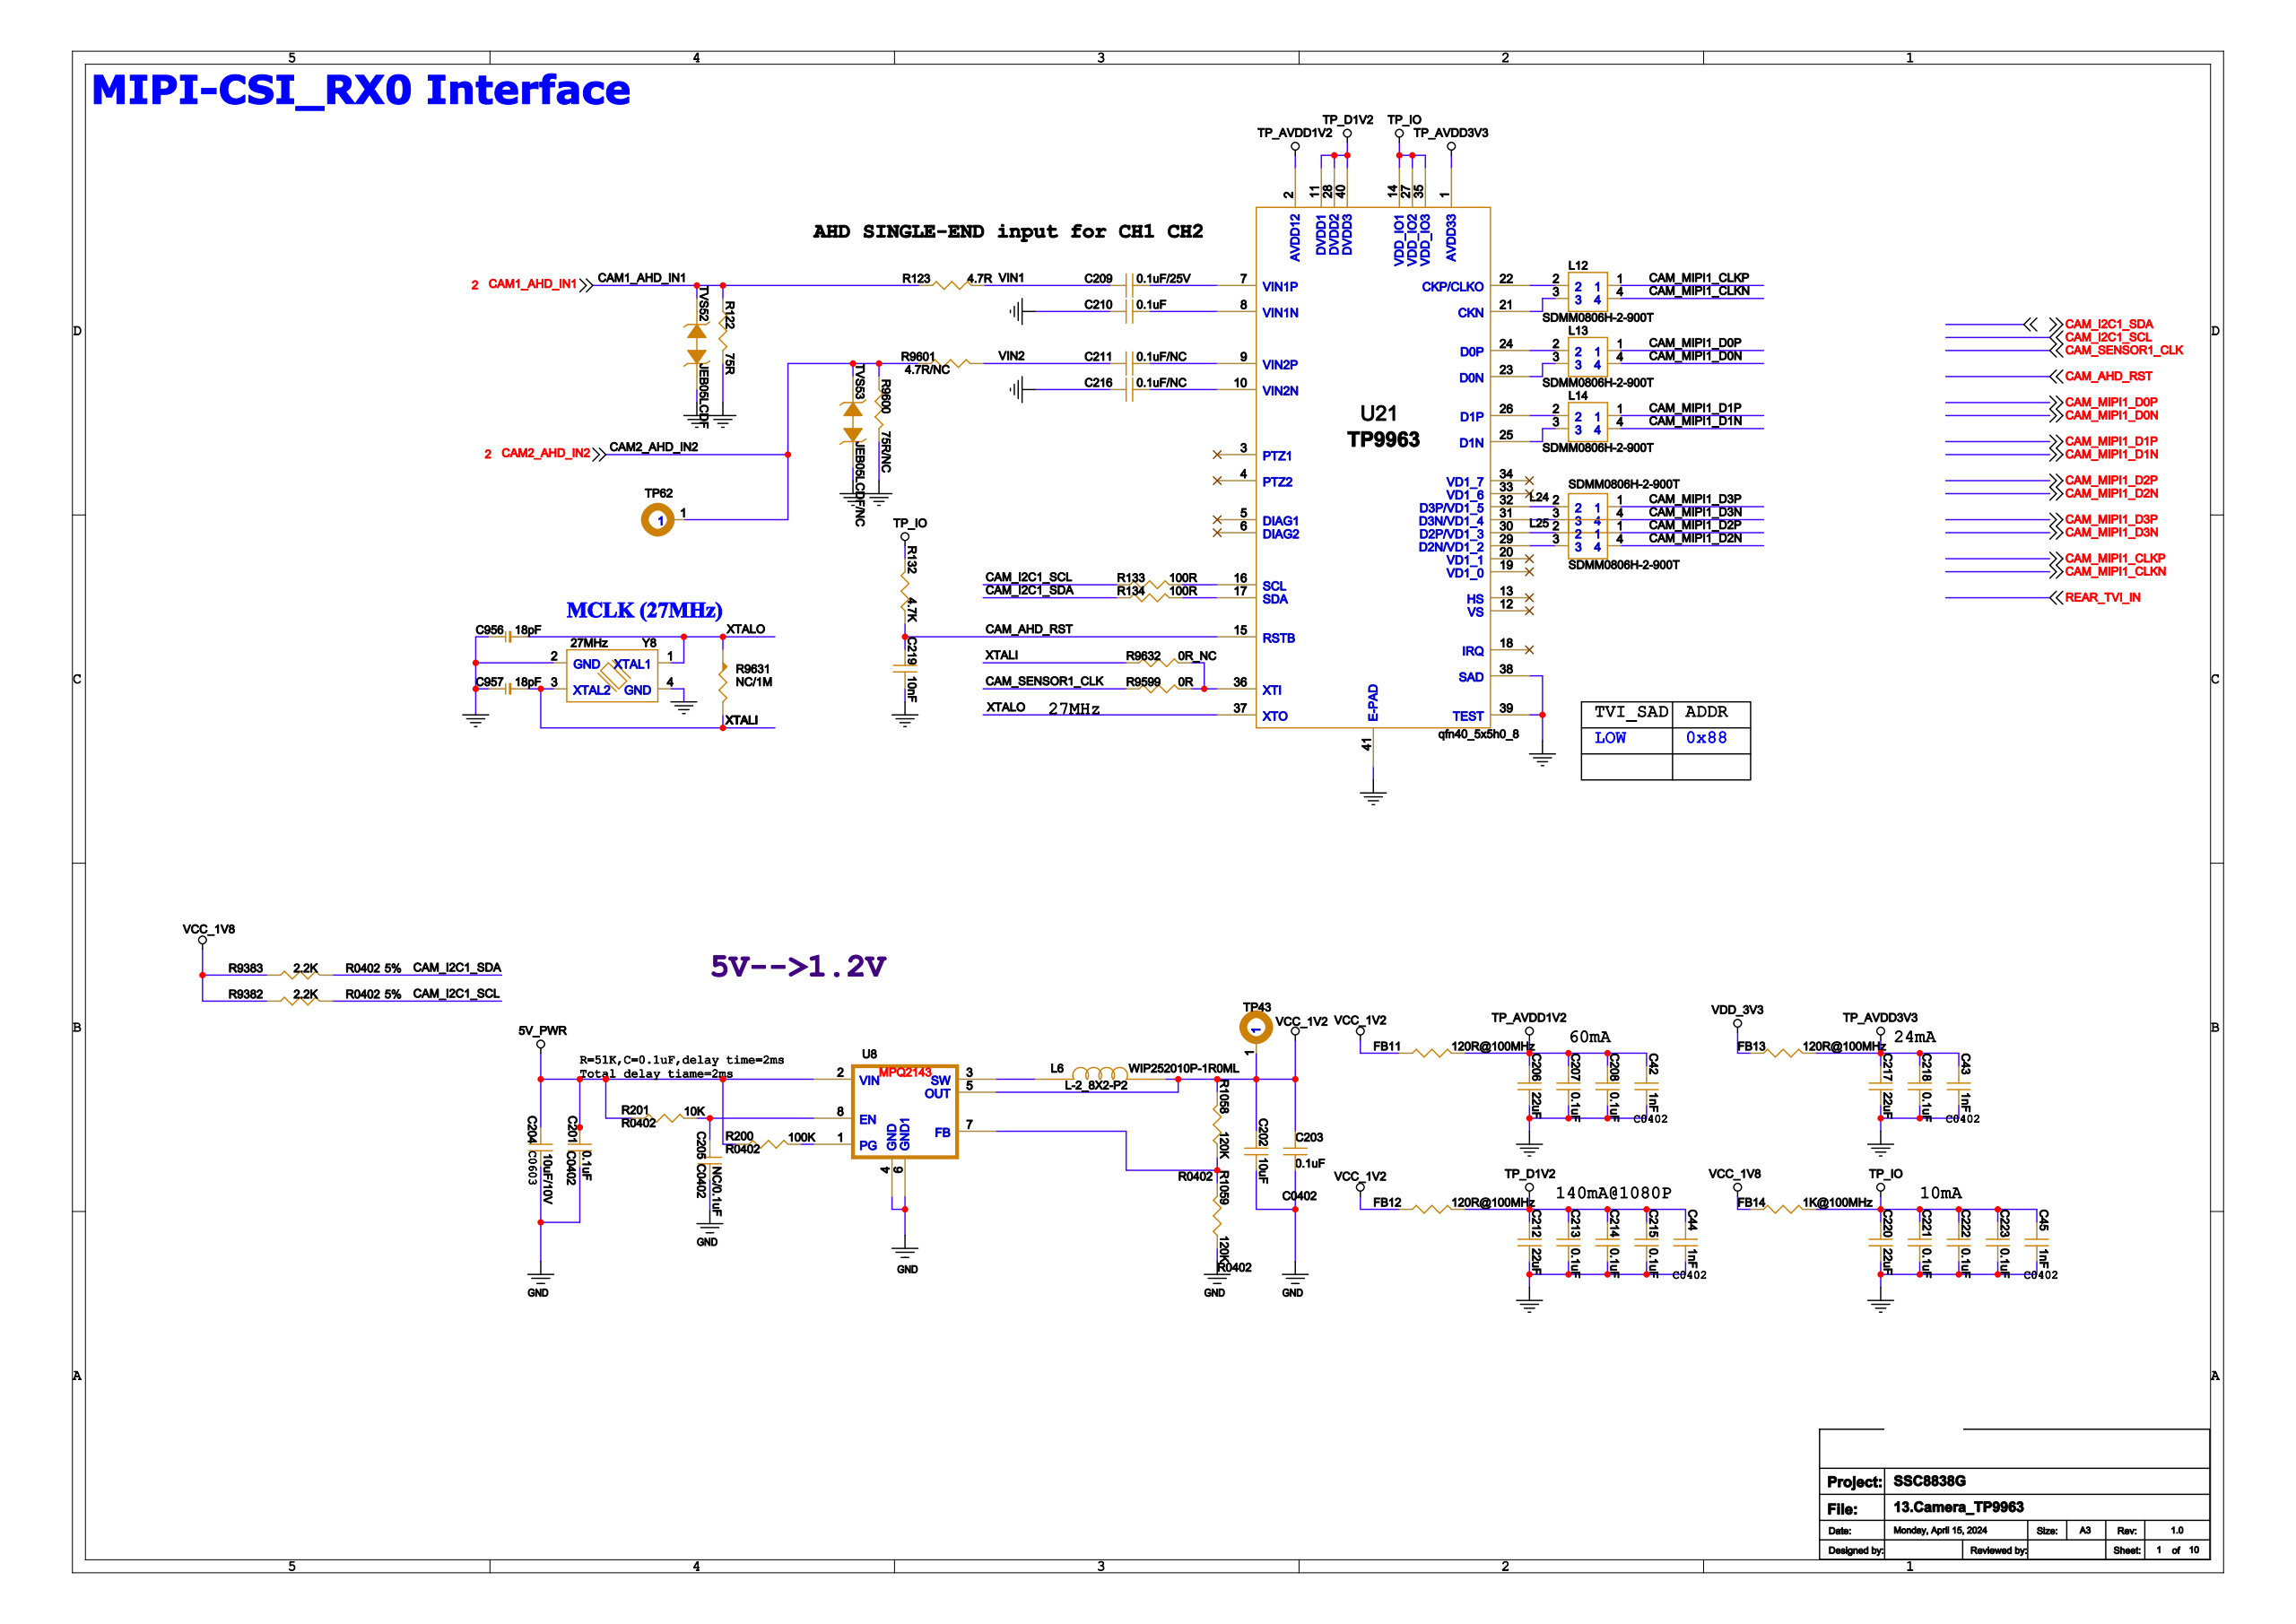Circuit board | Cadence Allegro | 958 parts | 601 nets | one sheet of the schematic
Parts on this sheet (reference | value | footprint):
C42 | 1nF | C0402
C43 | 1nF | C0402
C44 | 1nF | C0402
C45 | 1nF | C0402
C201 | 0.1uF | C0402
C202 | 10uF | C0603
C203 | 0.1uF | C0402
C204 | 10uF/10V | C0603
C205 | NC/0.1uF | C0402
C206 | 22uF | C0603
C207 | 0.1uF | C0402
C208 | 0.1uF | C0402
C209 | 0.1uF/25V | C0402
C210 | 0.1uF | C0402
C211 | 0.1uF/NC | C0402
C212 | 22uF | C0603
C213 | 0.1uF | C0402
C214 | 0.1uF | C0402
C215 | 0.1uF | C0402
C216 | 0.1uF/NC | C0402
C217 | 22uF | C0603
C218 | 0.1uF | C0402
C219 | 10nF | C0402
C220 | 22uF | C0603
C221 | 0.1uF | C0402
C222 | 0.1uF | C0402
C223 | 0.1uF | C0402
C956 | 18pF | C0402
C957 | 18pF | C0402
FB11 | 120R@100MHz | R0402
FB12 | 120R@100MHz | R0402
FB13 | 120R@100MHz | R0402
FB14 | 1K@100MHz | R0402
L6 | WIP252010P-1R0ML | L-2_8X2-P2
L12 | SDMM0806H-2-900T | ESD4_0_9X0_7H0
L13 | SDMM0806H-2-900T | ESD4_0_9X0_7H0
L14 | SDMM0806H-2-900T | ESD4_0_9X0_7H0
L24 | SDMM0806H-2-900T | ESD4_0_9X0_7H0
L25 | SDMM0806H-2-900T | ESD4_0_9X0_7H0
R122 | 75R | R0402
R123 | 4.7R | R0402
R132 | 4.7K | R0402
R133 | 100R | R0402
R134 | 100R | R0402
R200 | 100K | R0402
R201 | 10K | R0402
R1058 | 120K | R0402
R1059 | 120K | R0402
R9382 | 2.2K | R0402
R9383 | 2.2K | R0402
R9599 | 0R | R0402
R9600 | 75R/NC | R0402
R9601 | 4.7R/NC | R0402
R9631 | NC/1M | R0402
R9632 | 0R_NC | R0402
TP43 | HOLE | TP-C40
TP62 | HOLE | TP_0R50
TVS52 | JEB05LCDF | DFN1006
TVS53 | JEB05LCDF/NC | DFN1006
U8 | MPQ2143 | TSOT23-8
U21 | TP9963 | QFN40_5X5H0_8
Y8 | 27MHz | TCXO-3225
Nets of these parts (net: part-pin ...):
GND: C42-1 C43-1 C44-1 C45-1 C201-1 C202-1 C203-1 C204-1 C205-1 C206-1 C207-1 C208-1 C210-1 C212-1 C213-1 C214-1 C215-1 C216-1 C217-1 C218-1 C219-2 C220-1 C221-1 C222-1 C223-1 C956-1 C957-1 R122-1 R1059-1 R9600-1 TVS52-1 TVS53-1 U8-4 U8-6 Y8-2 Y8-4 U21-38 U21-39 U21-41
5V_PWR: C201-2 C204-2 R200-1 R201-1 U8-2
3V3_NORMAL: FB13-1
VCC_1V2: C202-2 C203-2 FB11-1 FB12-1 L6-2 R1058-2 TP43-1 U8-5
N21875047: C205-2 R201-2 U8-8
TP_AVDD1V2: C42-2 C206-2 C207-2 C208-2 FB11-2 U21-2
TP_D1V2: C44-2 C212-2 C213-2 C214-2 C215-2 FB12-2 U21-11 U21-28 U21-40
TP_AVDD3V3: C43-2 C217-2 C218-2 FB13-2 U21-1
TP_IO: C45-2 C220-2 C221-2 C222-2 C223-2 FB14-2 R132-2 U21-14 U21-27 U21-35
VIN1: C209-1 R123-1
N20987871: C209-2 U21-7
N20988210: C210-2 U21-8
VIN2: C211-1 R9601-1
N20987876: C211-2 U21-9
N20988212: C216-2 U21-10
CAM_AHD_RST: C219-1 R132-1 U21-15
XTALO_21205615: C956-2 R9631-1 Y8-1 U21-37
XTALI_21231710: C957-2 R9631-2 R9632-2 Y8-3
CAM_SENSOR1_CLK: R9599-2
1V8: FB14-1 R9382-1 R9383-1
CAM_MIPI1_CLKP: L12-1
N21456628: L12-2 U21-22
N21456631: L12-3 U21-21
CAM_MIPI1_CLKN: L12-4
CAM_MIPI1_D0P: L13-1
N21456634: L13-2 U21-24
N21456637: L13-3 U21-23
CAM_MIPI1_D0N: L13-4
CAM_MIPI1_D1P: L14-1
N21456640: L14-2 U21-26
N21456643: L14-3 U21-25
CAM_MIPI1_D1N: L14-4
CAM_MIPI1_D3P: L24-1
N21206676: L24-2 U21-32
N21206666: L24-3 U21-31
CAM_MIPI1_D3N: L24-4
CAM_MIPI1_D2P: L25-1
N21206739: L25-2 U21-30
N21206720: L25-3 U21-29
CAM_MIPI1_D2N: L25-4
N21875017: L6-1 U8-3
N21875067: R1058-1 R1059-2 U8-7
CAM1_AHD_IN1: R122-2 R123-2 TVS52-2
N20987744: R133-1 U21-16
CAM_I2C1_SCL: R133-2 R9382-2
N20987742: R134-1 U21-17
CAM_I2C1_SDA: R134-2 R9383-2
N21875104: R200-2 U8-1
N21232020: R9599-1 R9632-1 U21-36
CAM2_AHD_IN2: R9600-2 R9601-2 TP62-1 TVS53-2